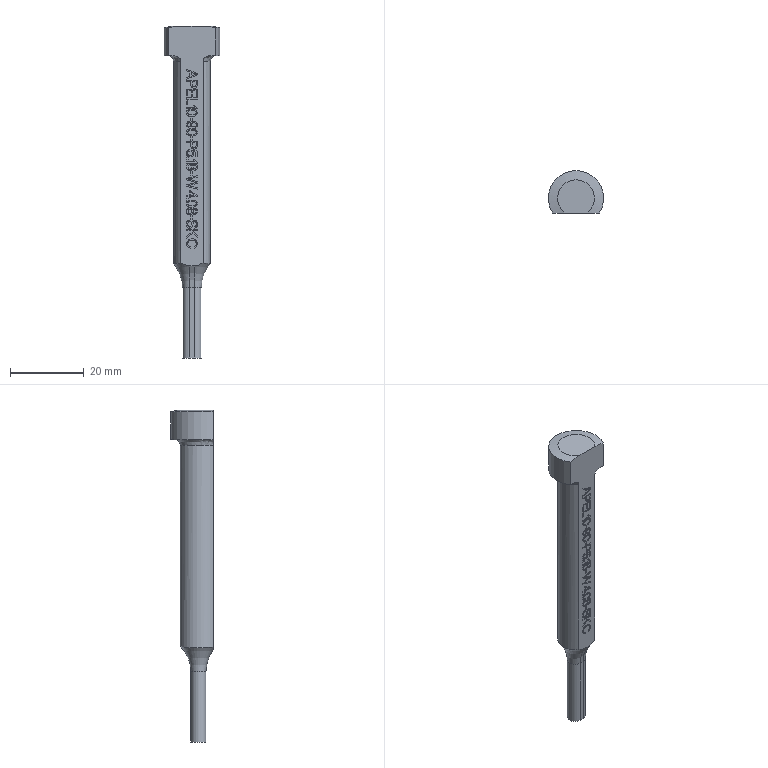Part | NX | features MI_APEL_0161 2 | 1 solid | 326 faces | box 15 x 11.5 x 90 mm | volume 5903 mm3 | plane 242 | cylinder 80 | torus 2 | spline 1 | cone 1 | commonest cylinder face diameters 0.936 x4 1.169 x4 1.393 x4 1.225 x3 1.462 x3 1.466 x3